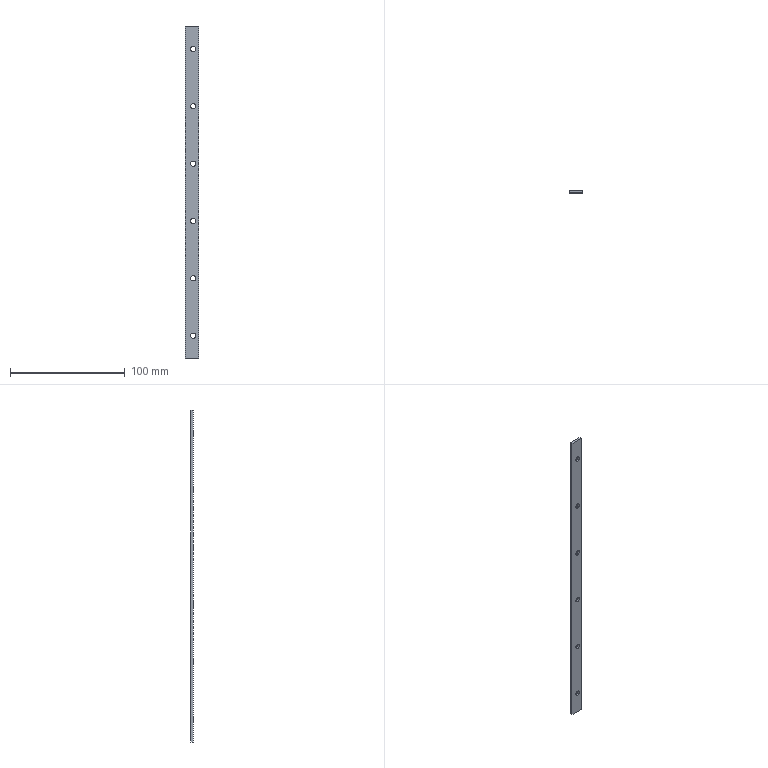Part | STEP file | Press strip (small) | 1 solid | 18 faces | box 12 x 2 x 289.5 mm | volume 6757 mm3 | cylinder 12 | plane 6 | commonest cylinder face diameters 4.5 x12
STEP:
#1=CARTESIAN_POINT('',(0.,0.,0.));
#2=DIRECTION('',(0.,0.,1.));
#3=DIRECTION('',(1.,0.,0.));
#4=AXIS2_PLACEMENT_3D('',#1,#2,#3);
#5=CARTESIAN_POINT('',(9.25,0.,19.5));
#6=VERTEX_POINT('',#5);
#7=CARTESIAN_POINT('',(9.25,-2.,19.5));
#8=VERTEX_POINT('',#7);
#9=CARTESIAN_POINT('',(9.25,0.001,19.5));
#10=DIRECTION('',(0.,-1.,0.));
#11=VECTOR('',#10,1.);
#12=LINE('',#9,#11);
#13=CARTESIAN_POINT('',(7.,0.001,19.5));
#14=DIRECTION('',(0.,-1.,0.));
#15=DIRECTION('',(1.,0.,0.));
#16=AXIS2_PLACEMENT_3D('',#13,#14,#15);
#17=CYLINDRICAL_SURFACE('',#16,2.25);
#18=CARTESIAN_POINT('',(6.283,0.));
#19=DIRECTION('',(0.,1.));
#20=VECTOR('',#19,1.);
#21=LINE('',#18,#20);
#22=(GEOMETRIC_REPRESENTATION_CONTEXT(2)PARAMETRIC_REPRESENTATION_CONTEXT()REPRESENTATION_CONTEXT('',''));
#23=DEFINITIONAL_REPRESENTATION('',(#21),#22);
#24=PCURVE('',#17,#23);
#25=CARTESIAN_POINT('',(7.,0.001,19.5));
#26=DIRECTION('',(0.,-1.,0.));
#27=DIRECTION('',(1.,0.,0.));
#28=AXIS2_PLACEMENT_3D('',#25,#26,#27);
#29=CYLINDRICAL_SURFACE('',#28,2.25);
#30=CARTESIAN_POINT('',(0.,0.));
#31=DIRECTION('',(0.,1.));
#32=VECTOR('',#31,1.);
#33=LINE('',#30,#32);
#34=(GEOMETRIC_REPRESENTATION_CONTEXT(2)PARAMETRIC_REPRESENTATION_CONTEXT()REPRESENTATION_CONTEXT('',''));
#35=DEFINITIONAL_REPRESENTATION('',(#33),#34);
#36=PCURVE('',#29,#35);
#37=SURFACE_CURVE('',#12,(#24,#36),.PCURVE_S1.);
#38=EDGE_CURVE('',#6,#8,#37,.T.);
#39=ORIENTED_EDGE('',*,*,#38,.T.);
#40=CARTESIAN_POINT('',(4.75,-2.,19.5));
#41=VERTEX_POINT('',#40);
#42=CARTESIAN_POINT('',(7.,-2.,19.5));
#43=DIRECTION('',(0.,-1.,0.));
#44=DIRECTION('',(1.,0.,0.));
#45=AXIS2_PLACEMENT_3D('',#42,#43,#44);
#46=CIRCLE('',#45,2.25);
#47=CARTESIAN_POINT('',(0.,2.001));
#48=DIRECTION('',(1.,0.));
#49=VECTOR('',#48,1.);
#50=LINE('',#47,#49);
#51=(GEOMETRIC_REPRESENTATION_CONTEXT(2)PARAMETRIC_REPRESENTATION_CONTEXT()REPRESENTATION_CONTEXT('',''));
#52=DEFINITIONAL_REPRESENTATION('',(#50),#51);
#53=PCURVE('',#17,#52);
#54=CARTESIAN_POINT('',(0.,-2.,289.5));
#55=DIRECTION('',(0.,1.,0.));
#56=DIRECTION('',(0.,0.,1.));
#57=AXIS2_PLACEMENT_3D('',#54,#55,#56);
#58=PLANE('',#57);
#59=CARTESIAN_POINT('',(-270.,9.25));
#60=CARTESIAN_POINT('',(-266.103,9.25));
#61=CARTESIAN_POINT('',(-268.051,5.875));
#62=CARTESIAN_POINT('',(-270.,2.5));
#63=CARTESIAN_POINT('',(-271.949,5.875));
#64=CARTESIAN_POINT('',(-273.897,9.25));
#65=CARTESIAN_POINT('',(-270.,9.25));
#66=(BOUNDED_CURVE()B_SPLINE_CURVE(2,(#59,#60,#61,#62,#63,#64,#65),.UNSPECIFIED.,.T.,.F.)B_SPLINE_CURVE_WITH_KNOTS((1,2,2,2,2,1),(-2.094,0.,2.094,4.189,6.283,8.378),.UNSPECIFIED.)CURVE()GEOMETRIC_REPRESENTATION_ITEM()RATIONAL_B_SPLINE_CURVE((1.,0.5,1.,0.5,1.,0.5,1.))REPRESENTATION_ITEM(''));
#67=(GEOMETRIC_REPRESENTATION_CONTEXT(2)PARAMETRIC_REPRESENTATION_CONTEXT()REPRESENTATION_CONTEXT('',''));
#68=DEFINITIONAL_REPRESENTATION('',(#66),#67);
#69=PCURVE('',#58,#68);
#70=SURFACE_CURVE('',#46,(#53,#69),.PCURVE_S1.);
#71=EDGE_CURVE('',#41,#8,#70,.T.);
#72=ORIENTED_EDGE('',*,*,#71,.F.);
#73=CARTESIAN_POINT('',(4.75,0.,19.5));
#74=VERTEX_POINT('',#73);
#75=CARTESIAN_POINT('',(4.75,0.001,19.5));
#76=DIRECTION('',(0.,-1.,0.));
#77=VECTOR('',#76,1.);
#78=LINE('',#75,#77);
#79=CARTESIAN_POINT('',(3.142,0.));
#80=DIRECTION('',(0.,1.));
#81=VECTOR('',#80,1.);
#82=LINE('',#79,#81);
#83=(GEOMETRIC_REPRESENTATION_CONTEXT(2)PARAMETRIC_REPRESENTATION_CONTEXT()REPRESENTATION_CONTEXT('',''));
#84=DEFINITIONAL_REPRESENTATION('',(#82),#83);
#85=PCURVE('',#17,#84);
#86=CARTESIAN_POINT('',(3.142,0.));
#87=DIRECTION('',(0.,1.));
#88=VECTOR('',#87,1.);
#89=LINE('',#86,#88);
#90=(GEOMETRIC_REPRESENTATION_CONTEXT(2)PARAMETRIC_REPRESENTATION_CONTEXT()REPRESENTATION_CONTEXT('',''));
#91=DEFINITIONAL_REPRESENTATION('',(#89),#90);
#92=PCURVE('',#29,#91);
#93=SURFACE_CURVE('',#78,(#85,#92),.PCURVE_S1.);
#94=EDGE_CURVE('',#74,#41,#93,.T.);
#95=ORIENTED_EDGE('',*,*,#94,.F.);
#96=CARTESIAN_POINT('',(7.,0.,19.5));
#97=DIRECTION('',(0.,-1.,0.));
#98=DIRECTION('',(1.,0.,0.));
#99=AXIS2_PLACEMENT_3D('',#96,#97,#98);
#100=CIRCLE('',#99,2.25);
#101=CARTESIAN_POINT('',(0.,0.001));
#102=DIRECTION('',(1.,0.));
#103=VECTOR('',#102,1.);
#104=LINE('',#101,#103);
#105=(GEOMETRIC_REPRESENTATION_CONTEXT(2)PARAMETRIC_REPRESENTATION_CONTEXT()REPRESENTATION_CONTEXT('',''));
#106=DEFINITIONAL_REPRESENTATION('',(#104),#105);
#107=PCURVE('',#17,#106);
#108=CARTESIAN_POINT('',(0.,0.,289.5));
#109=DIRECTION('',(0.,-1.,0.));
#110=DIRECTION('',(0.,0.,-1.));
#111=AXIS2_PLACEMENT_3D('',#108,#109,#110);
#112=PLANE('',#111);
#113=CARTESIAN_POINT('',(270.,7.));
#114=DIRECTION('',(0.,1.));
#115=AXIS2_PLACEMENT_2D('',#113,#114);
#116=CIRCLE('',#115,2.25);
#117=(GEOMETRIC_REPRESENTATION_CONTEXT(2)PARAMETRIC_REPRESENTATION_CONTEXT()REPRESENTATION_CONTEXT('',''));
#118=DEFINITIONAL_REPRESENTATION('',(#116),#117);
#119=PCURVE('',#112,#118);
#120=SURFACE_CURVE('',#100,(#107,#119),.PCURVE_S1.);
#121=EDGE_CURVE('',#74,#6,#120,.T.);
#122=ORIENTED_EDGE('',*,*,#121,.T.);
#123=EDGE_LOOP('',(#39,#72,#95,#122));
#124=FACE_BOUND('',#123,.F.);
#125=ADVANCED_FACE('',(#124),#17,.F.);
#126=CARTESIAN_POINT('',(9.25,0.,69.5));
#127=VERTEX_POINT('',#126);
#128=CARTESIAN_POINT('',(9.25,-2.,69.5));
#129=VERTEX_POINT('',#128);
#130=CARTESIAN_POINT('',(9.25,0.001,69.5));
#131=DIRECTION('',(0.,-1.,0.));
#132=VECTOR('',#131,1.);
#133=LINE('',#130,#132);
#134=CARTESIAN_POINT('',(7.,0.001,69.5));
#135=DIRECTION('',(0.,-1.,0.));
#136=DIRECTION('',(1.,0.,0.));
#137=AXIS2_PLACEMENT_3D('',#134,#135,#136);
#138=CYLINDRICAL_SURFACE('',#137,2.25);
#139=CARTESIAN_POINT('',(6.283,0.));
#140=DIRECTION('',(0.,1.));
#141=VECTOR('',#140,1.);
#142=LINE('',#139,#141);
#143=(GEOMETRIC_REPRESENTATION_CONTEXT(2)PARAMETRIC_REPRESENTATION_CONTEXT()REPRESENTATION_CONTEXT('',''));
#144=DEFINITIONAL_REPRESENTATION('',(#142),#143);
#145=PCURVE('',#138,#144);
#146=CARTESIAN_POINT('',(7.,0.001,69.5));
#147=DIRECTION('',(0.,-1.,0.));
#148=DIRECTION('',(1.,0.,0.));
#149=AXIS2_PLACEMENT_3D('',#146,#147,#148);
#150=CYLINDRICAL_SURFACE('',#149,2.25);
#151=CARTESIAN_POINT('',(0.,0.));
#152=DIRECTION('',(0.,1.));
#153=VECTOR('',#152,1.);
#154=LINE('',#151,#153);
#155=(GEOMETRIC_REPRESENTATION_CONTEXT(2)PARAMETRIC_REPRESENTATION_CONTEXT()REPRESENTATION_CONTEXT('',''));
#156=DEFINITIONAL_REPRESENTATION('',(#154),#155);
#157=PCURVE('',#150,#156);
#158=SURFACE_CURVE('',#133,(#145,#157),.PCURVE_S1.);
#159=EDGE_CURVE('',#127,#129,#158,.T.);
#160=ORIENTED_EDGE('',*,*,#159,.T.);
#161=CARTESIAN_POINT('',(4.75,-2.,69.5));
#162=VERTEX_POINT('',#161);
#163=CARTESIAN_POINT('',(7.,-2.,69.5));
#164=DIRECTION('',(0.,-1.,0.));
#165=DIRECTION('',(1.,0.,0.));
#166=AXIS2_PLACEMENT_3D('',#163,#164,#165);
#167=CIRCLE('',#166,2.25);
#168=CARTESIAN_POINT('',(0.,2.001));
#169=DIRECTION('',(1.,0.));
#170=VECTOR('',#169,1.);
#171=LINE('',#168,#170);
#172=(GEOMETRIC_REPRESENTATION_CONTEXT(2)PARAMETRIC_REPRESENTATION_CONTEXT()REPRESENTATION_CONTEXT('',''));
#173=DEFINITIONAL_REPRESENTATION('',(#171),#172);
#174=PCURVE('',#138,#173);
#175=CARTESIAN_POINT('',(-220.,9.25));
#176=CARTESIAN_POINT('',(-216.103,9.25));
#177=CARTESIAN_POINT('',(-218.051,5.875));
#178=CARTESIAN_POINT('',(-220.,2.5));
#179=CARTESIAN_POINT('',(-221.949,5.875));
#180=CARTESIAN_POINT('',(-223.897,9.25));
#181=CARTESIAN_POINT('',(-220.,9.25));
#182=(BOUNDED_CURVE()B_SPLINE_CURVE(2,(#175,#176,#177,#178,#179,#180,#181),.UNSPECIFIED.,.T.,.F.)B_SPLINE_CURVE_WITH_KNOTS((1,2,2,2,2,1),(-2.094,0.,2.094,4.189,6.283,8.378),.UNSPECIFIED.)CURVE()GEOMETRIC_REPRESENTATION_ITEM()RATIONAL_B_SPLINE_CURVE((1.,0.5,1.,0.5,1.,0.5,1.))REPRESENTATION_ITEM(''));
#183=(GEOMETRIC_REPRESENTATION_CONTEXT(2)PARAMETRIC_REPRESENTATION_CONTEXT()REPRESENTATION_CONTEXT('',''));
#184=DEFINITIONAL_REPRESENTATION('',(#182),#183);
#185=PCURVE('',#58,#184);
#186=SURFACE_CURVE('',#167,(#174,#185),.PCURVE_S1.);
#187=EDGE_CURVE('',#162,#129,#186,.T.);
#188=ORIENTED_EDGE('',*,*,#187,.F.);
#189=CARTESIAN_POINT('',(4.75,0.,69.5));
#190=VERTEX_POINT('',#189);
#191=CARTESIAN_POINT('',(4.75,0.001,69.5));
#192=DIRECTION('',(0.,-1.,0.));
#193=VECTOR('',#192,1.);
#194=LINE('',#191,#193);
#195=CARTESIAN_POINT('',(3.142,0.));
#196=DIRECTION('',(0.,1.));
#197=VECTOR('',#196,1.);
#198=LINE('',#195,#197);
#199=(GEOMETRIC_REPRESENTATION_CONTEXT(2)PARAMETRIC_REPRESENTATION_CONTEXT()REPRESENTATION_CONTEXT('',''));
#200=DEFINITIONAL_REPRESENTATION('',(#198),#199);
#201=PCURVE('',#138,#200);
#202=CARTESIAN_POINT('',(3.142,0.));
#203=DIRECTION('',(0.,1.));
#204=VECTOR('',#203,1.);
#205=LINE('',#202,#204);
#206=(GEOMETRIC_REPRESENTATION_CONTEXT(2)PARAMETRIC_REPRESENTATION_CONTEXT()REPRESENTATION_CONTEXT('',''));
#207=DEFINITIONAL_REPRESENTATION('',(#205),#206);
#208=PCURVE('',#150,#207);
#209=SURFACE_CURVE('',#194,(#201,#208),.PCURVE_S1.);
#210=EDGE_CURVE('',#190,#162,#209,.T.);
#211=ORIENTED_EDGE('',*,*,#210,.F.);
#212=CARTESIAN_POINT('',(7.,0.,69.5));
#213=DIRECTION('',(0.,-1.,0.));
#214=DIRECTION('',(1.,0.,0.));
#215=AXIS2_PLACEMENT_3D('',#212,#213,#214);
#216=CIRCLE('',#215,2.25);
#217=CARTESIAN_POINT('',(0.,0.001));
#218=DIRECTION('',(1.,0.));
#219=VECTOR('',#218,1.);
#220=LINE('',#217,#219);
#221=(GEOMETRIC_REPRESENTATION_CONTEXT(2)PARAMETRIC_REPRESENTATION_CONTEXT()REPRESENTATION_CONTEXT('',''));
#222=DEFINITIONAL_REPRESENTATION('',(#220),#221);
#223=PCURVE('',#138,#222);
#224=CARTESIAN_POINT('',(220.,7.));
#225=DIRECTION('',(0.,1.));
#226=AXIS2_PLACEMENT_2D('',#224,#225);
#227=CIRCLE('',#226,2.25);
#228=(GEOMETRIC_REPRESENTATION_CONTEXT(2)PARAMETRIC_REPRESENTATION_CONTEXT()REPRESENTATION_CONTEXT('',''));
#229=DEFINITIONAL_REPRESENTATION('',(#227),#228);
#230=PCURVE('',#112,#229);
#231=SURFACE_CURVE('',#216,(#223,#230),.PCURVE_S1.);
#232=EDGE_CURVE('',#190,#127,#231,.T.);
#233=ORIENTED_EDGE('',*,*,#232,.T.);
#234=EDGE_LOOP('',(#160,#188,#211,#233));
#235=FACE_BOUND('',#234,.F.);
#236=ADVANCED_FACE('',(#235),#138,.F.);
#237=CARTESIAN_POINT('',(9.25,0.,119.5));
#238=VERTEX_POINT('',#237);
#239=CARTESIAN_POINT('',(9.25,-2.,119.5));
#240=VERTEX_POINT('',#239);
#241=CARTESIAN_POINT('',(9.25,0.001,119.5));
#242=DIRECTION('',(0.,-1.,0.));
#243=VECTOR('',#242,1.);
#244=LINE('',#241,#243);
#245=CARTESIAN_POINT('',(7.,0.001,119.5));
#246=DIRECTION('',(0.,-1.,0.));
#247=DIRECTION('',(1.,0.,0.));
#248=AXIS2_PLACEMENT_3D('',#245,#246,#247);
#249=CYLINDRICAL_SURFACE('',#248,2.25);
#250=CARTESIAN_POINT('',(6.283,0.));
#251=DIRECTION('',(0.,1.));
#252=VECTOR('',#251,1.);
#253=LINE('',#250,#252);
#254=(GEOMETRIC_REPRESENTATION_CONTEXT(2)PARAMETRIC_REPRESENTATION_CONTEXT()REPRESENTATION_CONTEXT('',''));
#255=DEFINITIONAL_REPRESENTATION('',(#253),#254);
#256=PCURVE('',#249,#255);
#257=CARTESIAN_POINT('',(7.,0.001,119.5));
#258=DIRECTION('',(0.,-1.,0.));
#259=DIRECTION('',(1.,0.,0.));
#260=AXIS2_PLACEMENT_3D('',#257,#258,#259);
#261=CYLINDRICAL_SURFACE('',#260,2.25);
#262=CARTESIAN_POINT('',(0.,0.));
#263=DIRECTION('',(0.,1.));
#264=VECTOR('',#263,1.);
#265=LINE('',#262,#264);
#266=(GEOMETRIC_REPRESENTATION_CONTEXT(2)PARAMETRIC_REPRESENTATION_CONTEXT()REPRESENTATION_CONTEXT('',''));
#267=DEFINITIONAL_REPRESENTATION('',(#265),#266);
#268=PCURVE('',#261,#267);
#269=SURFACE_CURVE('',#244,(#256,#268),.PCURVE_S1.);
#270=EDGE_CURVE('',#238,#240,#269,.T.);
#271=ORIENTED_EDGE('',*,*,#270,.T.);
#272=CARTESIAN_POINT('',(4.75,-2.,119.5));
#273=VERTEX_POINT('',#272);
#274=CARTESIAN_POINT('',(7.,-2.,119.5));
#275=DIRECTION('',(0.,-1.,0.));
#276=DIRECTION('',(1.,0.,0.));
#277=AXIS2_PLACEMENT_3D('',#274,#275,#276);
#278=CIRCLE('',#277,2.25);
#279=CARTESIAN_POINT('',(0.,2.001));
#280=DIRECTION('',(1.,0.));
#281=VECTOR('',#280,1.);
#282=LINE('',#279,#281);
#283=(GEOMETRIC_REPRESENTATION_CONTEXT(2)PARAMETRIC_REPRESENTATION_CONTEXT()REPRESENTATION_CONTEXT('',''));
#284=DEFINITIONAL_REPRESENTATION('',(#282),#283);
#285=PCURVE('',#249,#284);
#286=CARTESIAN_POINT('',(-170.,9.25));
#287=CARTESIAN_POINT('',(-166.103,9.25));
#288=CARTESIAN_POINT('',(-168.051,5.875));
#289=CARTESIAN_POINT('',(-170.,2.5));
#290=CARTESIAN_POINT('',(-171.949,5.875));
#291=CARTESIAN_POINT('',(-173.897,9.25));
#292=CARTESIAN_POINT('',(-170.,9.25));
#293=(BOUNDED_CURVE()B_SPLINE_CURVE(2,(#286,#287,#288,#289,#290,#291,#292),.UNSPECIFIED.,.T.,.F.)B_SPLINE_CURVE_WITH_KNOTS((1,2,2,2,2,1),(-2.094,0.,2.094,4.189,6.283,8.378),.UNSPECIFIED.)CURVE()GEOMETRIC_REPRESENTATION_ITEM()RATIONAL_B_SPLINE_CURVE((1.,0.5,1.,0.5,1.,0.5,1.))REPRESENTATION_ITEM(''));
#294=(GEOMETRIC_REPRESENTATION_CONTEXT(2)PARAMETRIC_REPRESENTATION_CONTEXT()REPRESENTATION_CONTEXT('',''));
#295=DEFINITIONAL_REPRESENTATION('',(#293),#294);
#296=PCURVE('',#58,#295);
#297=SURFACE_CURVE('',#278,(#285,#296),.PCURVE_S1.);
#298=EDGE_CURVE('',#273,#240,#297,.T.);
#299=ORIENTED_EDGE('',*,*,#298,.F.);
#300=CARTESIAN_POINT('',(4.75,0.,119.5));
#301=VERTEX_POINT('',#300);
#302=CARTESIAN_POINT('',(4.75,0.001,119.5));
#303=DIRECTION('',(0.,-1.,0.));
#304=VECTOR('',#303,1.);
#305=LINE('',#302,#304);
#306=CARTESIAN_POINT('',(3.142,0.));
#307=DIRECTION('',(0.,1.));
#308=VECTOR('',#307,1.);
#309=LINE('',#306,#308);
#310=(GEOMETRIC_REPRESENTATION_CONTEXT(2)PARAMETRIC_REPRESENTATION_CONTEXT()REPRESENTATION_CONTEXT('',''));
#311=DEFINITIONAL_REPRESENTATION('',(#309),#310);
#312=PCURVE('',#249,#311);
#313=CARTESIAN_POINT('',(3.142,0.));
#314=DIRECTION('',(0.,1.));
#315=VECTOR('',#314,1.);
#316=LINE('',#313,#315);
#317=(GEOMETRIC_REPRESENTATION_CONTEXT(2)PARAMETRIC_REPRESENTATION_CONTEXT()REPRESENTATION_CONTEXT('',''));
#318=DEFINITIONAL_REPRESENTATION('',(#316),#317);
#319=PCURVE('',#261,#318);
#320=SURFACE_CURVE('',#305,(#312,#319),.PCURVE_S1.);
#321=EDGE_CURVE('',#301,#273,#320,.T.);
#322=ORIENTED_EDGE('',*,*,#321,.F.);
#323=CARTESIAN_POINT('',(7.,0.,119.5));
#324=DIRECTION('',(0.,-1.,0.));
#325=DIRECTION('',(1.,0.,0.));
#326=AXIS2_PLACEMENT_3D('',#323,#324,#325);
#327=CIRCLE('',#326,2.25);
#328=CARTESIAN_POINT('',(0.,0.001));
#329=DIRECTION('',(1.,0.));
#330=VECTOR('',#329,1.);
#331=LINE('',#328,#330);
#332=(GEOMETRIC_REPRESENTATION_CONTEXT(2)PARAMETRIC_REPRESENTATION_CONTEXT()REPRESENTATION_CONTEXT('',''));
#333=DEFINITIONAL_REPRESENTATION('',(#331),#332);
#334=PCURVE('',#249,#333);
#335=CARTESIAN_POINT('',(170.,7.));
#336=DIRECTION('',(0.,1.));
#337=AXIS2_PLACEMENT_2D('',#335,#336);
#338=CIRCLE('',#337,2.25);
#339=(GEOMETRIC_REPRESENTATION_CONTEXT(2)PARAMETRIC_REPRESENTATION_CONTEXT()REPRESENTATION_CONTEXT('',''));
#340=DEFINITIONAL_REPRESENTATION('',(#338),#339);
#341=PCURVE('',#112,#340);
#342=SURFACE_CURVE('',#327,(#334,#341),.PCURVE_S1.);
#343=EDGE_CURVE('',#301,#238,#342,.T.);
#344=ORIENTED_EDGE('',*,*,#343,.T.);
#345=EDGE_LOOP('',(#271,#299,#322,#344));
#346=FACE_BOUND('',#345,.F.);
#347=ADVANCED_FACE('',(#346),#249,.F.);
#348=CARTESIAN_POINT('',(9.25,0.,169.5));
#349=VERTEX_POINT('',#348);
#350=CARTESIAN_POINT('',(9.25,-2.,169.5));
#351=VERTEX_POINT('',#350);
#352=CARTESIAN_POINT('',(9.25,0.001,169.5));
#353=DIRECTION('',(0.,-1.,0.));
#354=VECTOR('',#353,1.);
#355=LINE('',#352,#354);
#356=CARTESIAN_POINT('',(7.,0.001,169.5));
#357=DIRECTION('',(0.,-1.,0.));
#358=DIRECTION('',(1.,0.,0.));
#359=AXIS2_PLACEMENT_3D('',#356,#357,#358);
#360=CYLINDRICAL_SURFACE('',#359,2.25);
#361=CARTESIAN_POINT('',(6.283,0.));
#362=DIRECTION('',(0.,1.));
#363=VECTOR('',#362,1.);
#364=LINE('',#361,#363);
#365=(GEOMETRIC_REPRESENTATION_CONTEXT(2)PARAMETRIC_REPRESENTATION_CONTEXT()REPRESENTATION_CONTEXT('',''));
#366=DEFINITIONAL_REPRESENTATION('',(#364),#365);
#367=PCURVE('',#360,#366);
#368=CARTESIAN_POINT('',(7.,0.001,169.5));
#369=DIRECTION('',(0.,-1.,0.));
#370=DIRECTION('',(1.,0.,0.));
#371=AXIS2_PLACEMENT_3D('',#368,#369,#370);
#372=CYLINDRICAL_SURFACE('',#371,2.25);
#373=CARTESIAN_POINT('',(0.,0.));
#374=DIRECTION('',(0.,1.));
#375=VECTOR('',#374,1.);
#376=LINE('',#373,#375);
#377=(GEOMETRIC_REPRESENTATION_CONTEXT(2)PARAMETRIC_REPRESENTATION_CONTEXT()REPRESENTATION_CONTEXT('',''));
#378=DEFINITIONAL_REPRESENTATION('',(#376),#377);
#379=PCURVE('',#372,#378);
#380=SURFACE_CURVE('',#355,(#367,#379),.PCURVE_S1.);
#381=EDGE_CURVE('',#349,#351,#380,.T.);
#382=ORIENTED_EDGE('',*,*,#381,.T.);
#383=CARTESIAN_POINT('',(4.75,-2.,169.5));
#384=VERTEX_POINT('',#383);
#385=CARTESIAN_POINT('',(7.,-2.,169.5));
#386=DIRECTION('',(0.,-1.,0.));
#387=DIRECTION('',(1.,0.,0.));
#388=AXIS2_PLACEMENT_3D('',#385,#386,#387);
#389=CIRCLE('',#388,2.25);
#390=CARTESIAN_POINT('',(0.,2.001));
#391=DIRECTION('',(1.,0.));
#392=VECTOR('',#391,1.);
#393=LINE('',#390,#392);
#394=(GEOMETRIC_REPRESENTATION_CONTEXT(2)PARAMETRIC_REPRESENTATION_CONTEXT()REPRESENTATION_CONTEXT('',''));
#395=DEFINITIONAL_REPRESENTATION('',(#393),#394);
#396=PCURVE('',#360,#395);
#397=CARTESIAN_POINT('',(-120.,9.25));
#398=CARTESIAN_POINT('',(-116.103,9.25));
#399=CARTESIAN_POINT('',(-118.051,5.875));
#400=CARTESIAN_POINT('',(-120.,2.5));
#401=CARTESIAN_POINT('',(-121.949,5.875));
#402=CARTESIAN_POINT('',(-123.897,9.25));
#403=CARTESIAN_POINT('',(-120.,9.25));
#404=(BOUNDED_CURVE()B_SPLINE_CURVE(2,(#397,#398,#399,#400,#401,#402,#403),.UNSPECIFIED.,.T.,.F.)B_SPLINE_CURVE_WITH_KNOTS((1,2,2,2,2,1),(-2.094,0.,2.094,4.189,6.283,8.378),.UNSPECIFIED.)CURVE()GEOMETRIC_REPRESENTATION_ITEM()RATIONAL_B_SPLINE_CURVE((1.,0.5,1.,0.5,1.,0.5,1.))REPRESENTATION_ITEM(''));
#405=(GEOMETRIC_REPRESENTATION_CONTEXT(2)PARAMETRIC_REPRESENTATION_CONTEXT()REPRESENTATION_CONTEXT('',''));
#406=DEFINITIONAL_REPRESENTATION('',(#404),#405);
#407=PCURVE('',#58,#406);
#408=SURFACE_CURVE('',#389,(#396,#407),.PCURVE_S1.);
#409=EDGE_CURVE('',#384,#351,#408,.T.);
#410=ORIENTED_EDGE('',*,*,#409,.F.);
#411=CARTESIAN_POINT('',(4.75,0.,169.5));
#412=VERTEX_POINT('',#411);
#413=CARTESIAN_POINT('',(4.75,0.001,169.5));
#414=DIRECTION('',(0.,-1.,0.));
#415=VECTOR('',#414,1.);
#416=LINE('',#413,#415);
#417=CARTESIAN_POINT('',(3.142,0.));
#418=DIRECTION('',(0.,1.));
#419=VECTOR('',#418,1.);
#420=LINE('',#417,#419);
#421=(GEOMETRIC_REPRESENTATION_CONTEXT(2)PARAMETRIC_REPRESENTATION_CONTEXT()REPRESENTATION_CONTEXT('',''));
#422=DEFINITIONAL_REPRESENTATION('',(#420),#421);
#423=PCURVE('',#360,#422);
#424=CARTESIAN_POINT('',(3.142,0.));
#425=DIRECTION('',(0.,1.));
#426=VECTOR('',#425,1.);
#427=LINE('',#424,#426);
#428=(GEOMETRIC_REPRESENTATION_CONTEXT(2)PARAMETRIC_REPRESENTATION_CONTEXT()REPRESENTATION_CONTEXT('',''));
#429=DEFINITIONAL_REPRESENTATION('',(#427),#428);
#430=PCURVE('',#372,#429);
#431=SURFACE_CURVE('',#416,(#423,#430),.PCURVE_S1.);
#432=EDGE_CURVE('',#412,#384,#431,.T.);
#433=ORIENTED_EDGE('',*,*,#432,.F.);
#434=CARTESIAN_POINT('',(7.,0.,169.5));
#435=DIRECTION('',(0.,-1.,0.));
#436=DIRECTION('',(1.,0.,0.));
#437=AXIS2_PLACEMENT_3D('',#434,#435,#436);
#438=CIRCLE('',#437,2.25);
#439=CARTESIAN_POINT('',(0.,0.001));
#440=DIRECTION('',(1.,0.));
#441=VECTOR('',#440,1.);
#442=LINE('',#439,#441);
#443=(GEOMETRIC_REPRESENTATION_CONTEXT(2)PARAMETRIC_REPRESENTATION_CONTEXT()REPRESENTATION_CONTEXT('',''));
#444=DEFINITIONAL_REPRESENTATION('',(#442),#443);
#445=PCURVE('',#360,#444);
#446=CARTESIAN_POINT('',(120.,7.));
#447=DIRECTION('',(0.,1.));
#448=AXIS2_PLACEMENT_2D('',#446,#447);
#449=CIRCLE('',#448,2.25);
#450=(GEOMETRIC_REPRESENTATION_CONTEXT(2)PARAMETRIC_REPRESENTATION_CONTEXT()REPRESENTATION_CONTEXT('',''));
#451=DEFINITIONAL_REPRESENTATION('',(#449),#450);
#452=PCURVE('',#112,#451);
#453=SURFACE_CURVE('',#438,(#445,#452),.PCURVE_S1.);
#454=EDGE_CURVE('',#412,#349,#453,.T.);
#455=ORIENTED_EDGE('',*,*,#454,.T.);
#456=EDGE_LOOP('',(#382,#410,#433,#455));
#457=FACE_BOUND('',#456,.F.);
#458=ADVANCED_FACE('',(#457),#360,.F.);
#459=CARTESIAN_POINT('',(9.25,0.,269.5));
#460=VERTEX_POINT('',#459);
#461=CARTESIAN_POINT('',(9.25,-2.,269.5));
#462=VERTEX_POINT('',#461);
#463=CARTESIAN_POINT('',(9.25,0.001,269.5));
#464=DIRECTION('',(0.,-1.,0.));
#465=VECTOR('',#464,1.);
#466=LINE('',#463,#465);
#467=CARTESIAN_POINT('',(7.,0.001,269.5));
#468=DIRECTION('',(0.,-1.,0.));
#469=DIRECTION('',(1.,0.,0.));
#470=AXIS2_PLACEMENT_3D('',#467,#468,#469);
#471=CYLINDRICAL_SURFACE('',#470,2.25);
#472=CARTESIAN_POINT('',(6.283,0.));
#473=DIRECTION('',(0.,1.));
#474=VECTOR('',#473,1.);
#475=LINE('',#472,#474);
#476=(GEOMETRIC_REPRESENTATION_CONTEXT(2)PARAMETRIC_REPRESENTATION_CONTEXT()REPRESENTATION_CONTEXT('',''));
#477=DEFINITIONAL_REPRESENTATION('',(#475),#476);
#478=PCURVE('',#471,#477);
#479=CARTESIAN_POINT('',(7.,0.001,269.5));
#480=DIRECTION('',(0.,-1.,0.));
#481=DIRECTION('',(1.,0.,0.));
#482=AXIS2_PLACEMENT_3D('',#479,#480,#481);
#483=CYLINDRICAL_SURFACE('',#482,2.25);
#484=CARTESIAN_POINT('',(0.,0.));
#485=DIRECTION('',(0.,1.));
#486=VECTOR('',#485,1.);
#487=LINE('',#484,#486);
#488=(GEOMETRIC_REPRESENTATION_CONTEXT(2)PARAMETRIC_REPRESENTATION_CONTEXT()REPRESENTATION_CONTEXT('',''));
#489=DEFINITIONAL_REPRESENTATION('',(#487),#488);
#490=PCURVE('',#483,#489);
#491=SURFACE_CURVE('',#466,(#478,#490),.PCURVE_S1.);
#492=EDGE_CURVE('',#460,#462,#491,.T.);
#493=ORIENTED_EDGE('',*,*,#492,.T.);
#494=CARTESIAN_POINT('',(4.75,-2.,269.5));
#495=VERTEX_POINT('',#494);
#496=CARTESIAN_POINT('',(7.,-2.,269.5));
#497=DIRECTION('',(0.,-1.,0.));
#498=DIRECTION('',(1.,0.,0.));
#499=AXIS2_PLACEMENT_3D('',#496,#497,#498);
#500=CIRCLE('',#499,2.25);
#501=CARTESIAN_POINT('',(0.,2.001));
#502=DIRECTION('',(1.,0.));
#503=VECTOR('',#502,1.);
#504=LINE('',#501,#503);
#505=(GEOMETRIC_REPRESENTATION_CONTEXT(2)PARAMETRIC_REPRESENTATION_CONTEXT()REPRESENTATION_CONTEXT('',''));
#506=DEFINITIONAL_REPRESENTATION('',(#504),#505);
#507=PCURVE('',#471,#506);
#508=CARTESIAN_POINT('',(-20.,9.25));
#509=CARTESIAN_POINT('',(-16.103,9.25));
#510=CARTESIAN_POINT('',(-18.051,5.875));
#511=CARTESIAN_POINT('',(-20.,2.5));
#512=CARTESIAN_POINT('',(-21.949,5.875));
#513=CARTESIAN_POINT('',(-23.897,9.25));
#514=CARTESIAN_POINT('',(-20.,9.25));
#515=(BOUNDED_CURVE()B_SPLINE_CURVE(2,(#508,#509,#510,#511,#512,#513,#514),.UNSPECIFIED.,.T.,.F.)B_SPLINE_CURVE_WITH_KNOTS((1,2,2,2,2,1),(-2.094,0.,2.094,4.189,6.283,8.378),.UNSPECIFIED.)CURVE()GEOMETRIC_REPRESENTATION_ITEM()RATIONAL_B_SPLINE_CURVE((1.,0.5,1.,0.5,1.,0.5,1.))REPRESENTATION_ITEM(''));
#516=(GEOMETRIC_REPRESENTATION_CONTEXT(2)PARAMETRIC_REPRESENTATION_CONTEXT()REPRESENTATION_CONTEXT('',''));
#517=DEFINITIONAL_REPRESENTATION('',(#515),#516);
#518=PCURVE('',#58,#517);
#519=SURFACE_CURVE('',#500,(#507,#518),.PCURVE_S1.);
#520=EDGE_CURVE('',#495,#462,#519,.T.);
#521=ORIENTED_EDGE('',*,*,#520,.F.);
#522=CARTESIAN_POINT('',(4.75,0.,269.5));
#523=VERTEX_POINT('',#522);
#524=CARTESIAN_POINT('',(4.75,0.001,269.5));
#525=DIRECTION('',(0.,-1.,0.));
#526=VECTOR('',#525,1.);
#527=LINE('',#524,#526);
#528=CARTESIAN_POINT('',(3.142,0.));
#529=DIRECTION('',(0.,1.));
#530=VECTOR('',#529,1.);
#531=LINE('',#528,#530);
#532=(GEOMETRIC_REPRESENTATION_CONTEXT(2)PARAMETRIC_REPRESENTATION_CONTEXT()REPRESENTATION_CONTEXT('',''));
#533=DEFINITIONAL_REPRESENTATION('',(#531),#532);
#534=PCURVE('',#471,#533);
#535=CARTESIAN_POINT('',(3.142,0.));
#536=DIRECTION('',(0.,1.));
#537=VECTOR('',#536,1.);
#538=LINE('',#535,#537);
#539=(GEOMETRIC_REPRESENTATION_CONTEXT(2)PARAMETRIC_REPRESENTATION_CONTEXT()REPRESENTATION_CONTEXT('',''));
#540=DEFINITIONAL_REPRESENTATION('',(#538),#539);
#541=PCURVE('',#483,#540);
#542=SURFACE_CURVE('',#527,(#534,#541),.PCURVE_S1.);
#543=EDGE_CURVE('',#523,#495,#542,.T.);
#544=ORIENTED_EDGE('',*,*,#543,.F.);
#545=CARTESIAN_POINT('',(7.,0.,269.5));
#546=DIRECTION('',(0.,-1.,0.));
#547=DIRECTION('',(1.,0.,0.));
#548=AXIS2_PLACEMENT_3D('',#545,#546,#547);
#549=CIRCLE('',#548,2.25);
#550=CARTESIAN_POINT('',(0.,0.001));
#551=DIRECTION('',(1.,0.));
#552=VECTOR('',#551,1.);
#553=LINE('',#550,#552);
#554=(GEOMETRIC_REPRESENTATION_CONTEXT(2)PARAMETRIC_REPRESENTATION_CONTEXT()REPRESENTATION_CONTEXT('',''));
#555=DEFINITIONAL_REPRESENTATION('',(#553),#554);
#556=PCURVE('',#471,#555);
#557=CARTESIAN_POINT('',(20.,7.));
#558=DIRECTION('',(0.,1.));
#559=AXIS2_PLACEMENT_2D('',#557,#558);
#560=CIRCLE('',#559,2.25);
#561=(GEOMETRIC_REPRESENTATION_CONTEXT(2)PARAMETRIC_REPRESENTATION_CONTEXT()REPRESENTATION_CONTEXT('',''));
#562=DEFINITIONAL_REPRESENTATION('',(#560),#561);
#563=PCURVE('',#112,#562);
#564=SURFACE_CURVE('',#549,(#556,#563),.PCURVE_S1.);
#565=EDGE_CURVE('',#523,#460,#564,.T.);
#566=ORIENTED_EDGE('',*,*,#565,.T.);
#567=EDGE_LOOP('',(#493,#521,#544,#566));
#568=FACE_BOUND('',#567,.F.);
#569=ADVANCED_FACE('',(#568),#471,.F.);
#570=CARTESIAN_POINT('',(9.25,0.,219.5));
#571=VERTEX_POINT('',#570);
#572=CARTESIAN_POINT('',(9.25,-2.,219.5));
#573=VERTEX_POINT('',#572);
#574=CARTESIAN_POINT('',(9.25,0.001,219.5));
#575=DIRECTION('',(0.,-1.,0.));
#576=VECTOR('',#575,1.);
#577=LINE('',#574,#576);
#578=CARTESIAN_POINT('',(7.,0.001,219.5));
#579=DIRECTION('',(0.,-1.,0.));
#580=DIRECTION('',(1.,0.,0.));
#581=AXIS2_PLACEMENT_3D('',#578,#579,#580);
#582=CYLINDRICAL_SURFACE('',#581,2.25);
#583=CARTESIAN_POINT('',(6.283,0.));
#584=DIRECTION('',(0.,1.));
#585=VECTOR('',#584,1.);
#586=LINE('',#583,#585);
#587=(GEOMETRIC_REPRESENTATION_CONTEXT(2)PARAMETRIC_REPRESENTATION_CONTEXT()REPRESENTATION_CONTEXT('',''));
#588=DEFINITIONAL_REPRESENTATION('',(#586),#587);
#589=PCURVE('',#582,#588);
#590=CARTESIAN_POINT('',(7.,0.001,219.5));
#591=DIRECTION('',(0.,-1.,0.));
#592=DIRECTION('',(1.,0.,0.));
#593=AXIS2_PLACEMENT_3D('',#590,#591,#592);
#594=CYLINDRICAL_SURFACE('',#593,2.25);
#595=CARTESIAN_POINT('',(0.,0.));
#596=DIRECTION('',(0.,1.));
#597=VECTOR('',#596,1.);
#598=LINE('',#595,#597);
#599=(GEOMETRIC_REPRESENTATION_CONTEXT(2)PARAMETRIC_REPRESENTATION_CONTEXT()REPRESENTATION_CONTEXT('',''));
#600=DEFINITIONAL_REPRESENTATION('',(#598),#599);
#601=PCURVE('',#594,#600);
#602=SURFACE_CURVE('',#577,(#589,#601),.PCURVE_S1.);
#603=EDGE_CURVE('',#571,#573,#602,.T.);
#604=ORIENTED_EDGE('',*,*,#603,.T.);
#605=CARTESIAN_POINT('',(4.75,-2.,219.5));
#606=VERTEX_POINT('',#605);
#607=CARTESIAN_POINT('',(7.,-2.,219.5));
#608=DIRECTION('',(0.,-1.,0.));
#609=DIRECTION('',(1.,0.,0.));
#610=AXIS2_PLACEMENT_3D('',#607,#608,#609);
#611=CIRCLE('',#610,2.25);
#612=CARTESIAN_POINT('',(0.,2.001));
#613=DIRECTION('',(1.,0.));
#614=VECTOR('',#613,1.);
#615=LINE('',#612,#614);
#616=(GEOMETRIC_REPRESENTATION_CONTEXT(2)PARAMETRIC_REPRESENTATION_CONTEXT()REPRESENTATION_CONTEXT('',''));
#617=DEFINITIONAL_REPRESENTATION('',(#615),#616);
#618=PCURVE('',#582,#617);
#619=CARTESIAN_POINT('',(-70.,9.25));
#620=CARTESIAN_POINT('',(-66.103,9.25));
#621=CARTESIAN_POINT('',(-68.051,5.875));
#622=CARTESIAN_POINT('',(-70.,2.5));
#623=CARTESIAN_POINT('',(-71.949,5.875));
#624=CARTESIAN_POINT('',(-73.897,9.25));
#625=CARTESIAN_POINT('',(-70.,9.25));
#626=(BOUNDED_CURVE()B_SPLINE_CURVE(2,(#619,#620,#621,#622,#623,#624,#625),.UNSPECIFIED.,.T.,.F.)B_SPLINE_CURVE_WITH_KNOTS((1,2,2,2,2,1),(-2.094,0.,2.094,4.189,6.283,8.378),.UNSPECIFIED.)CURVE()GEOMETRIC_REPRESENTATION_ITEM()RATIONAL_B_SPLINE_CURVE((1.,0.5,1.,0.5,1.,0.5,1.))REPRESENTATION_ITEM(''));
#627=(GEOMETRIC_REPRESENTATION_CONTEXT(2)PARAMETRIC_REPRESENTATION_CONTEXT()REPRESENTATION_CONTEXT('',''));
#628=DEFINITIONAL_REPRESENTATION('',(#626),#627);
#629=PCURVE('',#58,#628);
#630=SURFACE_CURVE('',#611,(#618,#629),.PCURVE_S1.);
#631=EDGE_CURVE('',#606,#573,#630,.T.);
#632=ORIENTED_EDGE('',*,*,#631,.F.);
#633=CARTESIAN_POINT('',(4.75,0.,219.5));
#634=VERTEX_POINT('',#633);
#635=CARTESIAN_POINT('',(4.75,0.001,219.5));
#636=DIRECTION('',(0.,-1.,0.));
#637=VECTOR('',#636,1.);
#638=LINE('',#635,#637);
#639=CARTESIAN_POINT('',(3.142,0.));
#640=DIRECTION('',(0.,1.));
#641=VECTOR('',#640,1.);
#642=LINE('',#639,#641);
#643=(GEOMETRIC_REPRESENTATION_CONTEXT(2)PARAMETRIC_REPRESENTATION_CONTEXT()REPRESENTATION_CONTEXT('',''));
#644=DEFINITIONAL_REPRESENTATION('',(#642),#643);
#645=PCURVE('',#582,#644);
#646=CARTESIAN_POINT('',(3.142,0.));
#647=DIRECTION('',(0.,1.));
#648=VECTOR('',#647,1.);
#649=LINE('',#646,#648);
#650=(GEOMETRIC_REPRESENTATION_CONTEXT(2)PARAMETRIC_REPRESENTATION_CONTEXT()REPRESENTATION_CONTEXT('',''));
#651=DEFINITIONAL_REPRESENTATION('',(#649),#650);
#652=PCURVE('',#594,#651);
#653=SURFACE_CURVE('',#638,(#645,#652),.PCURVE_S1.);
#654=EDGE_CURVE('',#634,#606,#653,.T.);
#655=ORIENTED_EDGE('',*,*,#654,.F.);
#656=CARTESIAN_POINT('',(7.,0.,219.5));
#657=DIRECTION('',(0.,-1.,0.));
#658=DIRECTION('',(1.,0.,0.));
#659=AXIS2_PLACEMENT_3D('',#656,#657,#658);
#660=CIRCLE('',#659,2.25);
#661=CARTESIAN_POINT('',(0.,0.001));
#662=DIRECTION('',(1.,0.));
#663=VECTOR('',#662,1.);
#664=LINE('',#661,#663);
#665=(GEOMETRIC_REPRESENTATION_CONTEXT(2)PARAMETRIC_REPRESENTATION_CONTEXT()REPRESENTATION_CONTEXT('',''));
#666=DEFINITIONAL_REPRESENTATION('',(#664),#665);
#667=PCURVE('',#582,#666);
#668=CARTESIAN_POINT('',(70.,7.));
#669=DIRECTION('',(0.,1.));
#670=AXIS2_PLACEMENT_2D('',#668,#669);
#671=CIRCLE('',#670,2.25);
#672=(GEOMETRIC_REPRESENTATION_CONTEXT(2)PARAMETRIC_REPRESENTATION_CONTEXT()REPRESENTATION_CONTEXT('',''));
#673=DEFINITIONAL_REPRESENTATION('',(#671),#672);
#674=PCURVE('',#112,#673);
#675=SURFACE_CURVE('',#660,(#667,#674),.PCURVE_S1.);
#676=EDGE_CURVE('',#634,#571,#675,.T.);
#677=ORIENTED_EDGE('',*,*,#676,.T.);
#678=EDGE_LOOP('',(#604,#632,#655,#677));
#679=FACE_BOUND('',#678,.F.);
#680=ADVANCED_FACE('',(#679),#582,.F.);
#681=CARTESIAN_POINT('',(7.,-2.,19.5));
#682=DIRECTION('',(0.,-1.,0.));
#683=DIRECTION('',(1.,0.,0.));
#684=AXIS2_PLACEMENT_3D('',#681,#682,#683);
#685=CIRCLE('',#684,2.25);
#686=CARTESIAN_POINT('',(-270.,9.25));
#687=CARTESIAN_POINT('',(-266.103,9.25));
#688=CARTESIAN_POINT('',(-268.051,5.875));
#689=CARTESIAN_POINT('',(-270.,2.5));
#690=CARTESIAN_POINT('',(-271.949,5.875));
#691=CARTESIAN_POINT('',(-273.897,9.25));
#692=CARTESIAN_POINT('',(-270.,9.25));
#693=(BOUNDED_CURVE()B_SPLINE_CURVE(2,(#686,#687,#688,#689,#690,#691,#692),.UNSPECIFIED.,.T.,.F.)B_SPLINE_CURVE_WITH_KNOTS((1,2,2,2,2,1),(-2.094,0.,2.094,4.189,6.283,8.378),.UNSPECIFIED.)CURVE()GEOMETRIC_REPRESENTATION_ITEM()RATIONAL_B_SPLINE_CURVE((1.,0.5,1.,0.5,1.,0.5,1.))REPRESENTATION_ITEM(''));
#694=(GEOMETRIC_REPRESENTATION_CONTEXT(2)PARAMETRIC_REPRESENTATION_CONTEXT()REPRESENTATION_CONTEXT('',''));
#695=DEFINITIONAL_REPRESENTATION('',(#693),#694);
#696=PCURVE('',#58,#695);
#697=CARTESIAN_POINT('',(0.,2.001));
#698=DIRECTION('',(1.,0.));
#699=VECTOR('',#698,1.);
#700=LINE('',#697,#699);
#701=(GEOMETRIC_REPRESENTATION_CONTEXT(2)PARAMETRIC_REPRESENTATION_CONTEXT()REPRESENTATION_CONTEXT('',''));
#702=DEFINITIONAL_REPRESENTATION('',(#700),#701);
#703=PCURVE('',#29,#702);
#704=SURFACE_CURVE('',#685,(#696,#703),.PCURVE_S1.);
#705=EDGE_CURVE('',#8,#41,#704,.T.);
#706=ORIENTED_EDGE('',*,*,#705,.F.);
#707=ORIENTED_EDGE('',*,*,#71,.F.);
#708=EDGE_LOOP('',(#706,#707));
#709=FACE_BOUND('',#708,.T.);
#710=CARTESIAN_POINT('',(7.,-2.,69.5));
#711=DIRECTION('',(0.,-1.,0.));
#712=DIRECTION('',(1.,0.,0.));
#713=AXIS2_PLACEMENT_3D('',#710,#711,#712);
#714=CIRCLE('',#713,2.25);
#715=CARTESIAN_POINT('',(-220.,9.25));
#716=CARTESIAN_POINT('',(-216.103,9.25));
#717=CARTESIAN_POINT('',(-218.051,5.875));
#718=CARTESIAN_POINT('',(-220.,2.5));
#719=CARTESIAN_POINT('',(-221.949,5.875));
#720=CARTESIAN_POINT('',(-223.897,9.25));
#721=CARTESIAN_POINT('',(-220.,9.25));
#722=(BOUNDED_CURVE()B_SPLINE_CURVE(2,(#715,#716,#717,#718,#719,#720,#721),.UNSPECIFIED.,.T.,.F.)B_SPLINE_CURVE_WITH_KNOTS((1,2,2,2,2,1),(-2.094,0.,2.094,4.189,6.283,8.378),.UNSPECIFIED.)CURVE()GEOMETRIC_REPRESENTATION_ITEM()RATIONAL_B_SPLINE_CURVE((1.,0.5,1.,0.5,1.,0.5,1.))REPRESENTATION_ITEM(''));
#723=(GEOMETRIC_REPRESENTATION_CONTEXT(2)PARAMETRIC_REPRESENTATION_CONTEXT()REPRESENTATION_CONTEXT('',''));
#724=DEFINITIONAL_REPRESENTATION('',(#722),#723);
#725=PCURVE('',#58,#724);
#726=CARTESIAN_POINT('',(0.,2.001));
#727=DIRECTION('',(1.,0.));
#728=VECTOR('',#727,1.);
#729=LINE('',#726,#728);
#730=(GEOMETRIC_REPRESENTATION_CONTEXT(2)PARAMETRIC_REPRESENTATION_CONTEXT()REPRESENTATION_CONTEXT('',''));
#731=DEFINITIONAL_REPRESENTATION('',(#729),#730);
#732=PCURVE('',#150,#731);
#733=SURFACE_CURVE('',#714,(#725,#732),.PCURVE_S1.);
#734=EDGE_CURVE('',#129,#162,#733,.T.);
#735=ORIENTED_EDGE('',*,*,#734,.F.);
#736=ORIENTED_EDGE('',*,*,#187,.F.);
#737=EDGE_LOOP('',(#735,#736));
#738=FACE_BOUND('',#737,.T.);
#739=CARTESIAN_POINT('',(7.,-2.,119.5));
#740=DIRECTION('',(0.,-1.,0.));
#741=DIRECTION('',(1.,0.,0.));
#742=AXIS2_PLACEMENT_3D('',#739,#740,#741);
#743=CIRCLE('',#742,2.25);
#744=CARTESIAN_POINT('',(-170.,9.25));
#745=CARTESIAN_POINT('',(-166.103,9.25));
#746=CARTESIAN_POINT('',(-168.051,5.875));
#747=CARTESIAN_POINT('',(-170.,2.5));
#748=CARTESIAN_POINT('',(-171.949,5.875));
#749=CARTESIAN_POINT('',(-173.897,9.25));
#750=CARTESIAN_POINT('',(-170.,9.25));
#751=(BOUNDED_CURVE()B_SPLINE_CURVE(2,(#744,#745,#746,#747,#748,#749,#750),.UNSPECIFIED.,.T.,.F.)B_SPLINE_CURVE_WITH_KNOTS((1,2,2,2,2,1),(-2.094,0.,2.094,4.189,6.283,8.378),.UNSPECIFIED.)CURVE()GEOMETRIC_REPRESENTATION_ITEM()RATIONAL_B_SPLINE_CURVE((1.,0.5,1.,0.5,1.,0.5,1.))REPRESENTATION_ITEM(''));
#752=(GEOMETRIC_REPRESENTATION_CONTEXT(2)PARAMETRIC_REPRESENTATION_CONTEXT()REPRESENTATION_CONTEXT('',''));
#753=DEFINITIONAL_REPRESENTATION('',(#751),#752);
#754=PCURVE('',#58,#753);
#755=CARTESIAN_POINT('',(0.,2.001));
#756=DIRECTION('',(1.,0.));
#757=VECTOR('',#756,1.);
#758=LINE('',#755,#757);
#759=(GEOMETRIC_REPRESENTATION_CONTEXT(2)PARAMETRIC_REPRESENTATION_CONTEXT()REPRESENTATION_CONTEXT('',''));
#760=DEFINITIONAL_REPRESENTATION('',(#758),#759);
#761=PCURVE('',#261,#760);
#762=SURFACE_CURVE('',#743,(#754,#761),.PCURVE_S1.);
#763=EDGE_CURVE('',#240,#273,#762,.T.);
#764=ORIENTED_EDGE('',*,*,#763,.F.);
#765=ORIENTED_EDGE('',*,*,#298,.F.);
#766=EDGE_LOOP('',(#764,#765));
#767=FACE_BOUND('',#766,.T.);
#768=CARTESIAN_POINT('',(7.,-2.,169.5));
#769=DIRECTION('',(0.,-1.,0.));
#770=DIRECTION('',(1.,0.,0.));
#771=AXIS2_PLACEMENT_3D('',#768,#769,#770);
#772=CIRCLE('',#771,2.25);
#773=CARTESIAN_POINT('',(-120.,9.25));
#774=CARTESIAN_POINT('',(-116.103,9.25));
#775=CARTESIAN_POINT('',(-118.051,5.875));
#776=CARTESIAN_POINT('',(-120.,2.5));
#777=CARTESIAN_POINT('',(-121.949,5.875));
#778=CARTESIAN_POINT('',(-123.897,9.25));
#779=CARTESIAN_POINT('',(-120.,9.25));
#780=(BOUNDED_CURVE()B_SPLINE_CURVE(2,(#773,#774,#775,#776,#777,#778,#779),.UNSPECIFIED.,.T.,.F.)B_SPLINE_CURVE_WITH_KNOTS((1,2,2,2,2,1),(-2.094,0.,2.094,4.189,6.283,8.378),.UNSPECIFIED.)CURVE()GEOMETRIC_REPRESENTATION_ITEM()RATIONAL_B_SPLINE_CURVE((1.,0.5,1.,0.5,1.,0.5,1.))REPRESENTATION_ITEM(''));
#781=(GEOMETRIC_REPRESENTATION_CONTEXT(2)PARAMETRIC_REPRESENTATION_CONTEXT()REPRESENTATION_CONTEXT('',''));
#782=DEFINITIONAL_REPRESENTATION('',(#780),#781);
#783=PCURVE('',#58,#782);
#784=CARTESIAN_POINT('',(0.,2.001));
#785=DIRECTION('',(1.,0.));
#786=VECTOR('',#785,1.);
#787=LINE('',#784,#786);
#788=(GEOMETRIC_REPRESENTATION_CONTEXT(2)PARAMETRIC_REPRESENTATION_CONTEXT()REPRESENTATION_CONTEXT('',''));
#789=DEFINITIONAL_REPRESENTATION('',(#787),#788);
#790=PCURVE('',#372,#789);
#791=SURFACE_CURVE('',#772,(#783,#790),.PCURVE_S1.);
#792=EDGE_CURVE('',#351,#384,#791,.T.);
#793=ORIENTED_EDGE('',*,*,#792,.F.);
#794=ORIENTED_EDGE('',*,*,#409,.F.);
#795=EDGE_LOOP('',(#793,#794));
#796=FACE_BOUND('',#795,.T.);
#797=CARTESIAN_POINT('',(12.,-2.,289.5));
#798=VERTEX_POINT('',#797);
#799=CARTESIAN_POINT('',(12.,-2.,0.));
#800=VERTEX_POINT('',#799);
#801=CARTESIAN_POINT('',(12.,-2.,289.5));
#802=DIRECTION('',(0.,0.,-1.));
#803=VECTOR('',#802,1.);
#804=LINE('',#801,#803);
#805=CARTESIAN_POINT('',(0.,12.));
#806=DIRECTION('',(-1.,0.));
#807=VECTOR('',#806,1.);
#808=LINE('',#805,#807);
#809=(GEOMETRIC_REPRESENTATION_CONTEXT(2)PARAMETRIC_REPRESENTATION_CONTEXT()REPRESENTATION_CONTEXT('',''));
#810=DEFINITIONAL_REPRESENTATION('',(#808),#809);
#811=PCURVE('',#58,#810);
#812=CARTESIAN_POINT('',(12.,0.,289.5));
#813=DIRECTION('',(-1.,0.,0.));
#814=DIRECTION('',(0.,0.,1.));
#815=AXIS2_PLACEMENT_3D('',#812,#813,#814);
#816=PLANE('',#815);
#817=CARTESIAN_POINT('',(0.,-2.));
#818=DIRECTION('',(-1.,0.));
#819=VECTOR('',#818,1.);
#820=LINE('',#817,#819);
#821=(GEOMETRIC_REPRESENTATION_CONTEXT(2)PARAMETRIC_REPRESENTATION_CONTEXT()REPRESENTATION_CONTEXT('',''));
#822=DEFINITIONAL_REPRESENTATION('',(#820),#821);
#823=PCURVE('',#816,#822);
#824=SURFACE_CURVE('',#804,(#811,#823),.PCURVE_S1.);
#825=EDGE_CURVE('',#798,#800,#824,.T.);
#826=ORIENTED_EDGE('',*,*,#825,.F.);
#827=CARTESIAN_POINT('',(0.,-2.,289.5));
#828=VERTEX_POINT('',#827);
#829=CARTESIAN_POINT('',(0.,-2.,289.5));
#830=DIRECTION('',(1.,0.,0.));
#831=VECTOR('',#830,1.);
#832=LINE('',#829,#831);
#833=CARTESIAN_POINT('',(0.,0.));
#834=DIRECTION('',(0.,1.));
#835=VECTOR('',#834,1.);
#836=LINE('',#833,#835);
#837=(GEOMETRIC_REPRESENTATION_CONTEXT(2)PARAMETRIC_REPRESENTATION_CONTEXT()REPRESENTATION_CONTEXT('',''));
#838=DEFINITIONAL_REPRESENTATION('',(#836),#837);
#839=PCURVE('',#58,#838);
#840=CARTESIAN_POINT('',(0.,-2.,289.5));
#841=DIRECTION('',(0.,0.,1.));
#842=DIRECTION('',(1.,0.,0.));
#843=AXIS2_PLACEMENT_3D('',#840,#841,#842);
#844=PLANE('',#843);
#845=CARTESIAN_POINT('',(0.,0.));
#846=DIRECTION('',(1.,0.));
#847=VECTOR('',#846,1.);
#848=LINE('',#845,#847);
#849=(GEOMETRIC_REPRESENTATION_CONTEXT(2)PARAMETRIC_REPRESENTATION_CONTEXT()REPRESENTATION_CONTEXT('',''));
#850=DEFINITIONAL_REPRESENTATION('',(#848),#849);
#851=PCURVE('',#844,#850);
#852=SURFACE_CURVE('',#832,(#839,#851),.PCURVE_S1.);
#853=EDGE_CURVE('',#828,#798,#852,.T.);
#854=ORIENTED_EDGE('',*,*,#853,.F.);
#855=CARTESIAN_POINT('',(0.,-2.,0.));
#856=VERTEX_POINT('',#855);
#857=CARTESIAN_POINT('',(0.,-2.,289.5));
#858=DIRECTION('',(0.,0.,1.));
#859=VECTOR('',#858,1.);
#860=LINE('',#857,#859);
#861=CARTESIAN_POINT('',(0.,0.));
#862=DIRECTION('',(1.,0.));
#863=VECTOR('',#862,1.);
#864=LINE('',#861,#863);
#865=(GEOMETRIC_REPRESENTATION_CONTEXT(2)PARAMETRIC_REPRESENTATION_CONTEXT()REPRESENTATION_CONTEXT('',''));
#866=DEFINITIONAL_REPRESENTATION('',(#864),#865);
#867=PCURVE('',#58,#866);
#868=CARTESIAN_POINT('',(0.,0.,289.5));
#869=DIRECTION('',(1.,0.,0.));
#870=DIRECTION('',(0.,1.,0.));
#871=AXIS2_PLACEMENT_3D('',#868,#869,#870);
#872=PLANE('',#871);
#873=CARTESIAN_POINT('',(-2.,0.));
#874=DIRECTION('',(0.,1.));
#875=VECTOR('',#874,1.);
#876=LINE('',#873,#875);
#877=(GEOMETRIC_REPRESENTATION_CONTEXT(2)PARAMETRIC_REPRESENTATION_CONTEXT()REPRESENTATION_CONTEXT('',''));
#878=DEFINITIONAL_REPRESENTATION('',(#876),#877);
#879=PCURVE('',#872,#878);
#880=SURFACE_CURVE('',#860,(#867,#879),.PCURVE_S1.);
#881=EDGE_CURVE('',#856,#828,#880,.T.);
#882=ORIENTED_EDGE('',*,*,#881,.F.);
#883=CARTESIAN_POINT('',(0.,-2.,0.));
#884=DIRECTION('',(-1.,0.,0.));
#885=VECTOR('',#884,1.);
#886=LINE('',#883,#885);
#887=CARTESIAN_POINT('',(-289.5,0.));
#888=DIRECTION('',(0.,-1.));
#889=VECTOR('',#888,1.);
#890=LINE('',#887,#889);
#891=(GEOMETRIC_REPRESENTATION_CONTEXT(2)PARAMETRIC_REPRESENTATION_CONTEXT()REPRESENTATION_CONTEXT('',''));
#892=DEFINITIONAL_REPRESENTATION('',(#890),#891);
#893=PCURVE('',#58,#892);
#894=CARTESIAN_POINT('',(0.,-2.,0.));
#895=DIRECTION('',(0.,0.,1.));
#896=DIRECTION('',(1.,0.,0.));
#897=AXIS2_PLACEMENT_3D('',#894,#895,#896);
#898=PLANE('',#897);
#899=CARTESIAN_POINT('',(0.,0.));
#900=DIRECTION('',(-1.,0.));
#901=VECTOR('',#900,1.);
#902=LINE('',#899,#901);
#903=(GEOMETRIC_REPRESENTATION_CONTEXT(2)PARAMETRIC_REPRESENTATION_CONTEXT()REPRESENTATION_CONTEXT('',''));
#904=DEFINITIONAL_REPRESENTATION('',(#902),#903);
#905=PCURVE('',#898,#904);
#906=SURFACE_CURVE('',#886,(#893,#905),.PCURVE_S1.);
#907=EDGE_CURVE('',#800,#856,#906,.T.);
#908=ORIENTED_EDGE('',*,*,#907,.F.);
#909=EDGE_LOOP('',(#826,#854,#882,#908));
#910=FACE_BOUND('',#909,.T.);
#911=CARTESIAN_POINT('',(7.,-2.,269.5));
#912=DIRECTION('',(0.,-1.,0.));
#913=DIRECTION('',(1.,0.,0.));
#914=AXIS2_PLACEMENT_3D('',#911,#912,#913);
#915=CIRCLE('',#914,2.25);
#916=CARTESIAN_POINT('',(-20.,9.25));
#917=CARTESIAN_POINT('',(-16.103,9.25));
#918=CARTESIAN_POINT('',(-18.051,5.875));
#919=CARTESIAN_POINT('',(-20.,2.5));
#920=CARTESIAN_POINT('',(-21.949,5.875));
#921=CARTESIAN_POINT('',(-23.897,9.25));
#922=CARTESIAN_POINT('',(-20.,9.25));
#923=(BOUNDED_CURVE()B_SPLINE_CURVE(2,(#916,#917,#918,#919,#920,#921,#922),.UNSPECIFIED.,.T.,.F.)B_SPLINE_CURVE_WITH_KNOTS((1,2,2,2,2,1),(-2.094,0.,2.094,4.189,6.283,8.378),.UNSPECIFIED.)CURVE()GEOMETRIC_REPRESENTATION_ITEM()RATIONAL_B_SPLINE_CURVE((1.,0.5,1.,0.5,1.,0.5,1.))REPRESENTATION_ITEM(''));
#924=(GEOMETRIC_REPRESENTATION_CONTEXT(2)PARAMETRIC_REPRESENTATION_CONTEXT()REPRESENTATION_CONTEXT('',''));
#925=DEFINITIONAL_REPRESENTATION('',(#923),#924);
#926=PCURVE('',#58,#925);
#927=CARTESIAN_POINT('',(0.,2.001));
#928=DIRECTION('',(1.,0.));
#929=VECTOR('',#928,1.);
#930=LINE('',#927,#929);
#931=(GEOMETRIC_REPRESENTATION_CONTEXT(2)PARAMETRIC_REPRESENTATION_CONTEXT()REPRESENTATION_CONTEXT('',''));
#932=DEFINITIONAL_REPRESENTATION('',(#930),#931);
#933=PCURVE('',#483,#932);
#934=SURFACE_CURVE('',#915,(#926,#933),.PCURVE_S1.);
#935=EDGE_CURVE('',#462,#495,#934,.T.);
#936=ORIENTED_EDGE('',*,*,#935,.F.);
#937=ORIENTED_EDGE('',*,*,#520,.F.);
#938=EDGE_LOOP('',(#936,#937));
#939=FACE_BOUND('',#938,.T.);
#940=CARTESIAN_POINT('',(7.,-2.,219.5));
#941=DIRECTION('',(0.,-1.,0.));
#942=DIRECTION('',(1.,0.,0.));
#943=AXIS2_PLACEMENT_3D('',#940,#941,#942);
#944=CIRCLE('',#943,2.25);
#945=CARTESIAN_POINT('',(-70.,9.25));
#946=CARTESIAN_POINT('',(-66.103,9.25));
#947=CARTESIAN_POINT('',(-68.051,5.875));
#948=CARTESIAN_POINT('',(-70.,2.5));
#949=CARTESIAN_POINT('',(-71.949,5.875));
#950=CARTESIAN_POINT('',(-73.897,9.25));
#951=CARTESIAN_POINT('',(-70.,9.25));
#952=(BOUNDED_CURVE()B_SPLINE_CURVE(2,(#945,#946,#947,#948,#949,#950,#951),.UNSPECIFIED.,.T.,.F.)B_SPLINE_CURVE_WITH_KNOTS((1,2,2,2,2,1),(-2.094,0.,2.094,4.189,6.283,8.378),.UNSPECIFIED.)CURVE()GEOMETRIC_REPRESENTATION_ITEM()RATIONAL_B_SPLINE_CURVE((1.,0.5,1.,0.5,1.,0.5,1.))REPRESENTATION_ITEM(''));
#953=(GEOMETRIC_REPRESENTATION_CONTEXT(2)PARAMETRIC_REPRESENTATION_CONTEXT()REPRESENTATION_CONTEXT('',''));
#954=DEFINITIONAL_REPRESENTATION('',(#952),#953);
#955=PCURVE('',#58,#954);
#956=CARTESIAN_POINT('',(0.,2.001));
#957=DIRECTION('',(1.,0.));
#958=VECTOR('',#957,1.);
#959=LINE('',#956,#958);
#960=(GEOMETRIC_REPRESENTATION_CONTEXT(2)PARAMETRIC_REPRESENTATION_CONTEXT()REPRESENTATION_CONTEXT('',''));
#961=DEFINITIONAL_REPRESENTATION('',(#959),#960);
#962=PCURVE('',#594,#961);
#963=SURFACE_CURVE('',#944,(#955,#962),.PCURVE_S1.);
#964=EDGE_CURVE('',#573,#606,#963,.T.);
#965=ORIENTED_EDGE('',*,*,#964,.F.);
#966=ORIENTED_EDGE('',*,*,#631,.F.);
#967=EDGE_LOOP('',(#965,#966));
#968=FACE_BOUND('',#967,.T.);
#969=ADVANCED_FACE('',(#709,#738,#767,#796,#910,#939,#968),#58,.F.);
#970=ORIENTED_EDGE('',*,*,#705,.F.);
#971=ORIENTED_EDGE('',*,*,#38,.F.);
#972=CARTESIAN_POINT('',(7.,0.,19.5));
#973=DIRECTION('',(0.,-1.,0.));
#974=DIRECTION('',(1.,0.,0.));
#975=AXIS2_PLACEMENT_3D('',#972,#973,#974);
#976=CIRCLE('',#975,2.25);
#977=CARTESIAN_POINT('',(0.,0.001));
#978=DIRECTION('',(1.,0.));
#979=VECTOR('',#978,1.);
#980=LINE('',#977,#979);
#981=(GEOMETRIC_REPRESENTATION_CONTEXT(2)PARAMETRIC_REPRESENTATION_CONTEXT()REPRESENTATION_CONTEXT('',''));
#982=DEFINITIONAL_REPRESENTATION('',(#980),#981);
#983=PCURVE('',#29,#982);
#984=CARTESIAN_POINT('',(270.,7.));
#985=DIRECTION('',(0.,1.));
#986=AXIS2_PLACEMENT_2D('',#984,#985);
#987=CIRCLE('',#986,2.25);
#988=(GEOMETRIC_REPRESENTATION_CONTEXT(2)PARAMETRIC_REPRESENTATION_CONTEXT()REPRESENTATION_CONTEXT('',''));
#989=DEFINITIONAL_REPRESENTATION('',(#987),#988);
#990=PCURVE('',#112,#989);
#991=SURFACE_CURVE('',#976,(#983,#990),.PCURVE_S1.);
#992=EDGE_CURVE('',#6,#74,#991,.T.);
#993=ORIENTED_EDGE('',*,*,#992,.T.);
#994=ORIENTED_EDGE('',*,*,#94,.T.);
#995=EDGE_LOOP('',(#970,#971,#993,#994));
#996=FACE_BOUND('',#995,.F.);
#997=ADVANCED_FACE('',(#996),#29,.F.);
#998=ORIENTED_EDGE('',*,*,#734,.F.);
#999=ORIENTED_EDGE('',*,*,#159,.F.);
#1000=CARTESIAN_POINT('',(7.,0.,69.5));
#1001=DIRECTION('',(0.,-1.,0.));
#1002=DIRECTION('',(1.,0.,0.));
#1003=AXIS2_PLACEMENT_3D('',#1000,#1001,#1002);
#1004=CIRCLE('',#1003,2.25);
#1005=CARTESIAN_POINT('',(0.,0.001));
#1006=DIRECTION('',(1.,0.));
#1007=VECTOR('',#1006,1.);
#1008=LINE('',#1005,#1007);
#1009=(GEOMETRIC_REPRESENTATION_CONTEXT(2)PARAMETRIC_REPRESENTATION_CONTEXT()REPRESENTATION_CONTEXT('',''));
#1010=DEFINITIONAL_REPRESENTATION('',(#1008),#1009);
#1011=PCURVE('',#150,#1010);
#1012=CARTESIAN_POINT('',(220.,7.));
#1013=DIRECTION('',(0.,1.));
#1014=AXIS2_PLACEMENT_2D('',#1012,#1013);
#1015=CIRCLE('',#1014,2.25);
#1016=(GEOMETRIC_REPRESENTATION_CONTEXT(2)PARAMETRIC_REPRESENTATION_CONTEXT()REPRESENTATION_CONTEXT('',''));
#1017=DEFINITIONAL_REPRESENTATION('',(#1015),#1016);
#1018=PCURVE('',#112,#1017);
#1019=SURFACE_CURVE('',#1004,(#1011,#1018),.PCURVE_S1.);
#1020=EDGE_CURVE('',#127,#190,#1019,.T.);
#1021=ORIENTED_EDGE('',*,*,#1020,.T.);
#1022=ORIENTED_EDGE('',*,*,#210,.T.);
#1023=EDGE_LOOP('',(#998,#999,#1021,#1022));
#1024=FACE_BOUND('',#1023,.F.);
#1025=ADVANCED_FACE('',(#1024),#150,.F.);
#1026=ORIENTED_EDGE('',*,*,#763,.F.);
#1027=ORIENTED_EDGE('',*,*,#270,.F.);
#1028=CARTESIAN_POINT('',(7.,0.,119.5));
#1029=DIRECTION('',(0.,-1.,0.));
#1030=DIRECTION('',(1.,0.,0.));
#1031=AXIS2_PLACEMENT_3D('',#1028,#1029,#1030);
#1032=CIRCLE('',#1031,2.25);
#1033=CARTESIAN_POINT('',(0.,0.001));
#1034=DIRECTION('',(1.,0.));
#1035=VECTOR('',#1034,1.);
#1036=LINE('',#1033,#1035);
#1037=(GEOMETRIC_REPRESENTATION_CONTEXT(2)PARAMETRIC_REPRESENTATION_CONTEXT()REPRESENTATION_CONTEXT('',''));
#1038=DEFINITIONAL_REPRESENTATION('',(#1036),#1037);
#1039=PCURVE('',#261,#1038);
#1040=CARTESIAN_POINT('',(170.,7.));
#1041=DIRECTION('',(0.,1.));
#1042=AXIS2_PLACEMENT_2D('',#1040,#1041);
#1043=CIRCLE('',#1042,2.25);
#1044=(GEOMETRIC_REPRESENTATION_CONTEXT(2)PARAMETRIC_REPRESENTATION_CONTEXT()REPRESENTATION_CONTEXT('',''));
#1045=DEFINITIONAL_REPRESENTATION('',(#1043),#1044);
#1046=PCURVE('',#112,#1045);
#1047=SURFACE_CURVE('',#1032,(#1039,#1046),.PCURVE_S1.);
#1048=EDGE_CURVE('',#238,#301,#1047,.T.);
#1049=ORIENTED_EDGE('',*,*,#1048,.T.);
#1050=ORIENTED_EDGE('',*,*,#321,.T.);
#1051=EDGE_LOOP('',(#1026,#1027,#1049,#1050));
#1052=FACE_BOUND('',#1051,.F.);
#1053=ADVANCED_FACE('',(#1052),#261,.F.);
#1054=ORIENTED_EDGE('',*,*,#792,.F.);
#1055=ORIENTED_EDGE('',*,*,#381,.F.);
#1056=CARTESIAN_POINT('',(7.,0.,169.5));
#1057=DIRECTION('',(0.,-1.,0.));
#1058=DIRECTION('',(1.,0.,0.));
#1059=AXIS2_PLACEMENT_3D('',#1056,#1057,#1058);
#1060=CIRCLE('',#1059,2.25);
#1061=CARTESIAN_POINT('',(0.,0.001));
#1062=DIRECTION('',(1.,0.));
#1063=VECTOR('',#1062,1.);
#1064=LINE('',#1061,#1063);
#1065=(GEOMETRIC_REPRESENTATION_CONTEXT(2)PARAMETRIC_REPRESENTATION_CONTEXT()REPRESENTATION_CONTEXT('',''));
#1066=DEFINITIONAL_REPRESENTATION('',(#1064),#1065);
#1067=PCURVE('',#372,#1066);
#1068=CARTESIAN_POINT('',(120.,7.));
#1069=DIRECTION('',(0.,1.));
#1070=AXIS2_PLACEMENT_2D('',#1068,#1069);
#1071=CIRCLE('',#1070,2.25);
#1072=(GEOMETRIC_REPRESENTATION_CONTEXT(2)PARAMETRIC_REPRESENTATION_CONTEXT()REPRESENTATION_CONTEXT('',''));
#1073=DEFINITIONAL_REPRESENTATION('',(#1071),#1072);
#1074=PCURVE('',#112,#1073);
#1075=SURFACE_CURVE('',#1060,(#1067,#1074),.PCURVE_S1.);
#1076=EDGE_CURVE('',#349,#412,#1075,.T.);
#1077=ORIENTED_EDGE('',*,*,#1076,.T.);
#1078=ORIENTED_EDGE('',*,*,#432,.T.);
#1079=EDGE_LOOP('',(#1054,#1055,#1077,#1078));
#1080=FACE_BOUND('',#1079,.F.);
#1081=ADVANCED_FACE('',(#1080),#372,.F.);
#1082=CARTESIAN_POINT('',(12.,0.,0.));
#1083=VERTEX_POINT('',#1082);
#1084=CARTESIAN_POINT('',(0.,0.,0.));
#1085=VERTEX_POINT('',#1084);
#1086=CARTESIAN_POINT('',(0.,0.,0.));
#1087=DIRECTION('',(-1.,0.,0.));
#1088=VECTOR('',#1087,1.);
#1089=LINE('',#1086,#1088);
#1090=CARTESIAN_POINT('',(0.,2.));
#1091=DIRECTION('',(-1.,0.));
#1092=VECTOR('',#1091,1.);
#1093=LINE('',#1090,#1092);
#1094=(GEOMETRIC_REPRESENTATION_CONTEXT(2)PARAMETRIC_REPRESENTATION_CONTEXT()REPRESENTATION_CONTEXT('',''));
#1095=DEFINITIONAL_REPRESENTATION('',(#1093),#1094);
#1096=PCURVE('',#898,#1095);
#1097=CARTESIAN_POINT('',(289.5,0.));
#1098=DIRECTION('',(0.,-1.));
#1099=VECTOR('',#1098,1.);
#1100=LINE('',#1097,#1099);
#1101=(GEOMETRIC_REPRESENTATION_CONTEXT(2)PARAMETRIC_REPRESENTATION_CONTEXT()REPRESENTATION_CONTEXT('',''));
#1102=DEFINITIONAL_REPRESENTATION('',(#1100),#1101);
#1103=PCURVE('',#112,#1102);
#1104=SURFACE_CURVE('',#1089,(#1096,#1103),.PCURVE_S1.);
#1105=EDGE_CURVE('',#1083,#1085,#1104,.T.);
#1106=ORIENTED_EDGE('',*,*,#1105,.F.);
#1107=CARTESIAN_POINT('',(12.,-2.,0.));
#1108=DIRECTION('',(0.,1.,0.));
#1109=VECTOR('',#1108,1.);
#1110=LINE('',#1107,#1109);
#1111=CARTESIAN_POINT('',(12.,0.));
#1112=DIRECTION('',(0.,1.));
#1113=VECTOR('',#1112,1.);
#1114=LINE('',#1111,#1113);
#1115=(GEOMETRIC_REPRESENTATION_CONTEXT(2)PARAMETRIC_REPRESENTATION_CONTEXT()REPRESENTATION_CONTEXT('',''));
#1116=DEFINITIONAL_REPRESENTATION('',(#1114),#1115);
#1117=PCURVE('',#898,#1116);
#1118=CARTESIAN_POINT('',(-289.5,-2.));
#1119=DIRECTION('',(0.,1.));
#1120=VECTOR('',#1119,1.);
#1121=LINE('',#1118,#1120);
#1122=(GEOMETRIC_REPRESENTATION_CONTEXT(2)PARAMETRIC_REPRESENTATION_CONTEXT()REPRESENTATION_CONTEXT('',''));
#1123=DEFINITIONAL_REPRESENTATION('',(#1121),#1122);
#1124=PCURVE('',#816,#1123);
#1125=SURFACE_CURVE('',#1110,(#1117,#1124),.PCURVE_S1.);
#1126=EDGE_CURVE('',#800,#1083,#1125,.T.);
#1127=ORIENTED_EDGE('',*,*,#1126,.F.);
#1128=ORIENTED_EDGE('',*,*,#907,.T.);
#1129=CARTESIAN_POINT('',(0.,-2.,0.));
#1130=DIRECTION('',(0.,-1.,0.));
#1131=VECTOR('',#1130,1.);
#1132=LINE('',#1129,#1131);
#1133=CARTESIAN_POINT('',(0.,0.));
#1134=DIRECTION('',(0.,-1.));
#1135=VECTOR('',#1134,1.);
#1136=LINE('',#1133,#1135);
#1137=(GEOMETRIC_REPRESENTATION_CONTEXT(2)PARAMETRIC_REPRESENTATION_CONTEXT()REPRESENTATION_CONTEXT('',''));
#1138=DEFINITIONAL_REPRESENTATION('',(#1136),#1137);
#1139=PCURVE('',#898,#1138);
#1140=CARTESIAN_POINT('',(-2.,-289.5));
#1141=DIRECTION('',(-1.,0.));
#1142=VECTOR('',#1141,1.);
#1143=LINE('',#1140,#1142);
#1144=(GEOMETRIC_REPRESENTATION_CONTEXT(2)PARAMETRIC_REPRESENTATION_CONTEXT()REPRESENTATION_CONTEXT('',''));
#1145=DEFINITIONAL_REPRESENTATION('',(#1143),#1144);
#1146=PCURVE('',#872,#1145);
#1147=SURFACE_CURVE('',#1132,(#1139,#1146),.PCURVE_S1.);
#1148=EDGE_CURVE('',#1085,#856,#1147,.T.);
#1149=ORIENTED_EDGE('',*,*,#1148,.F.);
#1150=EDGE_LOOP('',(#1106,#1127,#1128,#1149));
#1151=FACE_BOUND('',#1150,.T.);
#1152=ADVANCED_FACE('',(#1151),#898,.F.);
#1153=CARTESIAN_POINT('',(12.,0.,289.5));
#1154=VERTEX_POINT('',#1153);
#1155=CARTESIAN_POINT('',(12.,0.,289.5));
#1156=DIRECTION('',(0.,0.,-1.));
#1157=VECTOR('',#1156,1.);
#1158=LINE('',#1155,#1157);
#1159=CARTESIAN_POINT('',(0.,0.));
#1160=DIRECTION('',(-1.,0.));
#1161=VECTOR('',#1160,1.);
#1162=LINE('',#1159,#1161);
#1163=(GEOMETRIC_REPRESENTATION_CONTEXT(2)PARAMETRIC_REPRESENTATION_CONTEXT()REPRESENTATION_CONTEXT('',''));
#1164=DEFINITIONAL_REPRESENTATION('',(#1162),#1163);
#1165=PCURVE('',#816,#1164);
#1166=CARTESIAN_POINT('',(0.,12.));
#1167=DIRECTION('',(1.,0.));
#1168=VECTOR('',#1167,1.);
#1169=LINE('',#1166,#1168);
#1170=(GEOMETRIC_REPRESENTATION_CONTEXT(2)PARAMETRIC_REPRESENTATION_CONTEXT()REPRESENTATION_CONTEXT('',''));
#1171=DEFINITIONAL_REPRESENTATION('',(#1169),#1170);
#1172=PCURVE('',#112,#1171);
#1173=SURFACE_CURVE('',#1158,(#1165,#1172),.PCURVE_S1.);
#1174=EDGE_CURVE('',#1154,#1083,#1173,.T.);
#1175=ORIENTED_EDGE('',*,*,#1174,.F.);
#1176=CARTESIAN_POINT('',(12.,0.,289.5));
#1177=DIRECTION('',(0.,1.,0.));
#1178=VECTOR('',#1177,1.);
#1179=LINE('',#1176,#1178);
#1180=CARTESIAN_POINT('',(0.,0.));
#1181=DIRECTION('',(0.,1.));
#1182=VECTOR('',#1181,1.);
#1183=LINE('',#1180,#1182);
#1184=(GEOMETRIC_REPRESENTATION_CONTEXT(2)PARAMETRIC_REPRESENTATION_CONTEXT()REPRESENTATION_CONTEXT('',''));
#1185=DEFINITIONAL_REPRESENTATION('',(#1183),#1184);
#1186=PCURVE('',#816,#1185);
#1187=CARTESIAN_POINT('',(12.,2.));
#1188=DIRECTION('',(0.,1.));
#1189=VECTOR('',#1188,1.);
#1190=LINE('',#1187,#1189);
#1191=(GEOMETRIC_REPRESENTATION_CONTEXT(2)PARAMETRIC_REPRESENTATION_CONTEXT()REPRESENTATION_CONTEXT('',''));
#1192=DEFINITIONAL_REPRESENTATION('',(#1190),#1191);
#1193=PCURVE('',#844,#1192);
#1194=SURFACE_CURVE('',#1179,(#1186,#1193),.PCURVE_S1.);
#1195=EDGE_CURVE('',#798,#1154,#1194,.T.);
#1196=ORIENTED_EDGE('',*,*,#1195,.F.);
#1197=ORIENTED_EDGE('',*,*,#825,.T.);
#1198=ORIENTED_EDGE('',*,*,#1126,.T.);
#1199=EDGE_LOOP('',(#1175,#1196,#1197,#1198));
#1200=FACE_BOUND('',#1199,.T.);
#1201=ADVANCED_FACE('',(#1200),#816,.F.);
#1202=ORIENTED_EDGE('',*,*,#1195,.T.);
#1203=CARTESIAN_POINT('',(0.,0.,289.5));
#1204=VERTEX_POINT('',#1203);
#1205=CARTESIAN_POINT('',(0.,0.,289.5));
#1206=DIRECTION('',(-1.,0.,0.));
#1207=VECTOR('',#1206,1.);
#1208=LINE('',#1205,#1207);
#1209=CARTESIAN_POINT('',(0.,2.));
#1210=DIRECTION('',(-1.,0.));
#1211=VECTOR('',#1210,1.);
#1212=LINE('',#1209,#1211);
#1213=(GEOMETRIC_REPRESENTATION_CONTEXT(2)PARAMETRIC_REPRESENTATION_CONTEXT()REPRESENTATION_CONTEXT('',''));
#1214=DEFINITIONAL_REPRESENTATION('',(#1212),#1213);
#1215=PCURVE('',#844,#1214);
#1216=CARTESIAN_POINT('',(0.,0.));
#1217=DIRECTION('',(0.,-1.));
#1218=VECTOR('',#1217,1.);
#1219=LINE('',#1216,#1218);
#1220=(GEOMETRIC_REPRESENTATION_CONTEXT(2)PARAMETRIC_REPRESENTATION_CONTEXT()REPRESENTATION_CONTEXT('',''));
#1221=DEFINITIONAL_REPRESENTATION('',(#1219),#1220);
#1222=PCURVE('',#112,#1221);
#1223=SURFACE_CURVE('',#1208,(#1215,#1222),.PCURVE_S1.);
#1224=EDGE_CURVE('',#1154,#1204,#1223,.T.);
#1225=ORIENTED_EDGE('',*,*,#1224,.T.);
#1226=CARTESIAN_POINT('',(0.,-2.,289.5));
#1227=DIRECTION('',(0.,-1.,0.));
#1228=VECTOR('',#1227,1.);
#1229=LINE('',#1226,#1228);
#1230=CARTESIAN_POINT('',(0.,0.));
#1231=DIRECTION('',(0.,-1.));
#1232=VECTOR('',#1231,1.);
#1233=LINE('',#1230,#1232);
#1234=(GEOMETRIC_REPRESENTATION_CONTEXT(2)PARAMETRIC_REPRESENTATION_CONTEXT()REPRESENTATION_CONTEXT('',''));
#1235=DEFINITIONAL_REPRESENTATION('',(#1233),#1234);
#1236=PCURVE('',#844,#1235);
#1237=CARTESIAN_POINT('',(-2.,0.));
#1238=DIRECTION('',(-1.,0.));
#1239=VECTOR('',#1238,1.);
#1240=LINE('',#1237,#1239);
#1241=(GEOMETRIC_REPRESENTATION_CONTEXT(2)PARAMETRIC_REPRESENTATION_CONTEXT()REPRESENTATION_CONTEXT('',''));
#1242=DEFINITIONAL_REPRESENTATION('',(#1240),#1241);
#1243=PCURVE('',#872,#1242);
#1244=SURFACE_CURVE('',#1229,(#1236,#1243),.PCURVE_S1.);
#1245=EDGE_CURVE('',#1204,#828,#1244,.T.);
#1246=ORIENTED_EDGE('',*,*,#1245,.T.);
#1247=ORIENTED_EDGE('',*,*,#853,.T.);
#1248=EDGE_LOOP('',(#1202,#1225,#1246,#1247));
#1249=FACE_BOUND('',#1248,.T.);
#1250=ADVANCED_FACE('',(#1249),#844,.T.);
#1251=ORIENTED_EDGE('',*,*,#881,.T.);
#1252=ORIENTED_EDGE('',*,*,#1245,.F.);
#1253=CARTESIAN_POINT('',(0.,0.,289.5));
#1254=DIRECTION('',(0.,0.,1.));
#1255=VECTOR('',#1254,1.);
#1256=LINE('',#1253,#1255);
#1257=CARTESIAN_POINT('',(0.,0.));
#1258=DIRECTION('',(0.,1.));
#1259=VECTOR('',#1258,1.);
#1260=LINE('',#1257,#1259);
#1261=(GEOMETRIC_REPRESENTATION_CONTEXT(2)PARAMETRIC_REPRESENTATION_CONTEXT()REPRESENTATION_CONTEXT('',''));
#1262=DEFINITIONAL_REPRESENTATION('',(#1260),#1261);
#1263=PCURVE('',#872,#1262);
#1264=CARTESIAN_POINT('',(0.,0.));
#1265=DIRECTION('',(-1.,0.));
#1266=VECTOR('',#1265,1.);
#1267=LINE('',#1264,#1266);
#1268=(GEOMETRIC_REPRESENTATION_CONTEXT(2)PARAMETRIC_REPRESENTATION_CONTEXT()REPRESENTATION_CONTEXT('',''));
#1269=DEFINITIONAL_REPRESENTATION('',(#1267),#1268);
#1270=PCURVE('',#112,#1269);
#1271=SURFACE_CURVE('',#1256,(#1263,#1270),.PCURVE_S1.);
#1272=EDGE_CURVE('',#1085,#1204,#1271,.T.);
#1273=ORIENTED_EDGE('',*,*,#1272,.F.);
#1274=ORIENTED_EDGE('',*,*,#1148,.T.);
#1275=EDGE_LOOP('',(#1251,#1252,#1273,#1274));
#1276=FACE_BOUND('',#1275,.T.);
#1277=ADVANCED_FACE('',(#1276),#872,.F.);
#1278=ORIENTED_EDGE('',*,*,#935,.F.);
#1279=ORIENTED_EDGE('',*,*,#492,.F.);
#1280=CARTESIAN_POINT('',(7.,0.,269.5));
#1281=DIRECTION('',(0.,-1.,0.));
#1282=DIRECTION('',(1.,0.,0.));
#1283=AXIS2_PLACEMENT_3D('',#1280,#1281,#1282);
#1284=CIRCLE('',#1283,2.25);
#1285=CARTESIAN_POINT('',(0.,0.001));
#1286=DIRECTION('',(1.,0.));
#1287=VECTOR('',#1286,1.);
#1288=LINE('',#1285,#1287);
#1289=(GEOMETRIC_REPRESENTATION_CONTEXT(2)PARAMETRIC_REPRESENTATION_CONTEXT()REPRESENTATION_CONTEXT('',''));
#1290=DEFINITIONAL_REPRESENTATION('',(#1288),#1289);
#1291=PCURVE('',#483,#1290);
#1292=CARTESIAN_POINT('',(20.,7.));
#1293=DIRECTION('',(0.,1.));
#1294=AXIS2_PLACEMENT_2D('',#1292,#1293);
#1295=CIRCLE('',#1294,2.25);
#1296=(GEOMETRIC_REPRESENTATION_CONTEXT(2)PARAMETRIC_REPRESENTATION_CONTEXT()REPRESENTATION_CONTEXT('',''));
#1297=DEFINITIONAL_REPRESENTATION('',(#1295),#1296);
#1298=PCURVE('',#112,#1297);
#1299=SURFACE_CURVE('',#1284,(#1291,#1298),.PCURVE_S1.);
#1300=EDGE_CURVE('',#460,#523,#1299,.T.);
#1301=ORIENTED_EDGE('',*,*,#1300,.T.);
#1302=ORIENTED_EDGE('',*,*,#543,.T.);
#1303=EDGE_LOOP('',(#1278,#1279,#1301,#1302));
#1304=FACE_BOUND('',#1303,.F.);
#1305=ADVANCED_FACE('',(#1304),#483,.F.);
#1306=ORIENTED_EDGE('',*,*,#964,.F.);
#1307=ORIENTED_EDGE('',*,*,#603,.F.);
#1308=CARTESIAN_POINT('',(7.,0.,219.5));
#1309=DIRECTION('',(0.,-1.,0.));
#1310=DIRECTION('',(1.,0.,0.));
#1311=AXIS2_PLACEMENT_3D('',#1308,#1309,#1310);
#1312=CIRCLE('',#1311,2.25);
#1313=CARTESIAN_POINT('',(0.,0.001));
#1314=DIRECTION('',(1.,0.));
#1315=VECTOR('',#1314,1.);
#1316=LINE('',#1313,#1315);
#1317=(GEOMETRIC_REPRESENTATION_CONTEXT(2)PARAMETRIC_REPRESENTATION_CONTEXT()REPRESENTATION_CONTEXT('',''));
#1318=DEFINITIONAL_REPRESENTATION('',(#1316),#1317);
#1319=PCURVE('',#594,#1318);
#1320=CARTESIAN_POINT('',(70.,7.));
#1321=DIRECTION('',(0.,1.));
#1322=AXIS2_PLACEMENT_2D('',#1320,#1321);
#1323=CIRCLE('',#1322,2.25);
#1324=(GEOMETRIC_REPRESENTATION_CONTEXT(2)PARAMETRIC_REPRESENTATION_CONTEXT()REPRESENTATION_CONTEXT('',''));
#1325=DEFINITIONAL_REPRESENTATION('',(#1323),#1324);
#1326=PCURVE('',#112,#1325);
#1327=SURFACE_CURVE('',#1312,(#1319,#1326),.PCURVE_S1.);
#1328=EDGE_CURVE('',#571,#634,#1327,.T.);
#1329=ORIENTED_EDGE('',*,*,#1328,.T.);
#1330=ORIENTED_EDGE('',*,*,#654,.T.);
#1331=EDGE_LOOP('',(#1306,#1307,#1329,#1330));
#1332=FACE_BOUND('',#1331,.F.);
#1333=ADVANCED_FACE('',(#1332),#594,.F.);
#1334=ORIENTED_EDGE('',*,*,#992,.T.);
#1335=ORIENTED_EDGE('',*,*,#121,.T.);
#1336=EDGE_LOOP('',(#1334,#1335));
#1337=FACE_BOUND('',#1336,.T.);
#1338=ORIENTED_EDGE('',*,*,#1020,.T.);
#1339=ORIENTED_EDGE('',*,*,#232,.T.);
#1340=EDGE_LOOP('',(#1338,#1339));
#1341=FACE_BOUND('',#1340,.T.);
#1342=ORIENTED_EDGE('',*,*,#1048,.T.);
#1343=ORIENTED_EDGE('',*,*,#343,.T.);
#1344=EDGE_LOOP('',(#1342,#1343));
#1345=FACE_BOUND('',#1344,.T.);
#1346=ORIENTED_EDGE('',*,*,#1076,.T.);
#1347=ORIENTED_EDGE('',*,*,#454,.T.);
#1348=EDGE_LOOP('',(#1346,#1347));
#1349=FACE_BOUND('',#1348,.T.);
#1350=ORIENTED_EDGE('',*,*,#1272,.T.);
#1351=ORIENTED_EDGE('',*,*,#1224,.F.);
#1352=ORIENTED_EDGE('',*,*,#1174,.T.);
#1353=ORIENTED_EDGE('',*,*,#1105,.T.);
#1354=EDGE_LOOP('',(#1350,#1351,#1352,#1353));
#1355=FACE_BOUND('',#1354,.T.);
#1356=ORIENTED_EDGE('',*,*,#1300,.T.);
#1357=ORIENTED_EDGE('',*,*,#565,.T.);
#1358=EDGE_LOOP('',(#1356,#1357));
#1359=FACE_BOUND('',#1358,.T.);
#1360=ORIENTED_EDGE('',*,*,#1328,.T.);
#1361=ORIENTED_EDGE('',*,*,#676,.T.);
#1362=EDGE_LOOP('',(#1360,#1361));
#1363=FACE_BOUND('',#1362,.T.);
#1364=ADVANCED_FACE('',(#1337,#1341,#1345,#1349,#1355,#1359,#1363),#112,.F.);
#1365=CLOSED_SHELL('',(#125,#236,#347,#458,#569,#680,#969,#997,#1025,#1053,#1081,#1152,#1201,#1250,#1277,#1305,#1333,#1364));
#1366=MANIFOLD_SOLID_BREP('',#1365);
#1367=(LENGTH_UNIT()NAMED_UNIT(*)SI_UNIT(.MILLI.,.METRE.));
#1368=UNCERTAINTY_MEASURE_WITH_UNIT(LENGTH_MEASURE(0.0000001),#1367,'','');
#1369=(NAMED_UNIT(*)PLANE_ANGLE_UNIT()SI_UNIT($,.RADIAN.));
#1370=(NAMED_UNIT(*)SI_UNIT($,.STERADIAN.)SOLID_ANGLE_UNIT());
#1371=(GEOMETRIC_REPRESENTATION_CONTEXT(3)GLOBAL_UNCERTAINTY_ASSIGNED_CONTEXT((#1368))GLOBAL_UNIT_ASSIGNED_CONTEXT((#1367,#1369,#1370))REPRESENTATION_CONTEXT('',''));
#1372=ADVANCED_BREP_SHAPE_REPRESENTATION('',(#4,#1366),#1371);